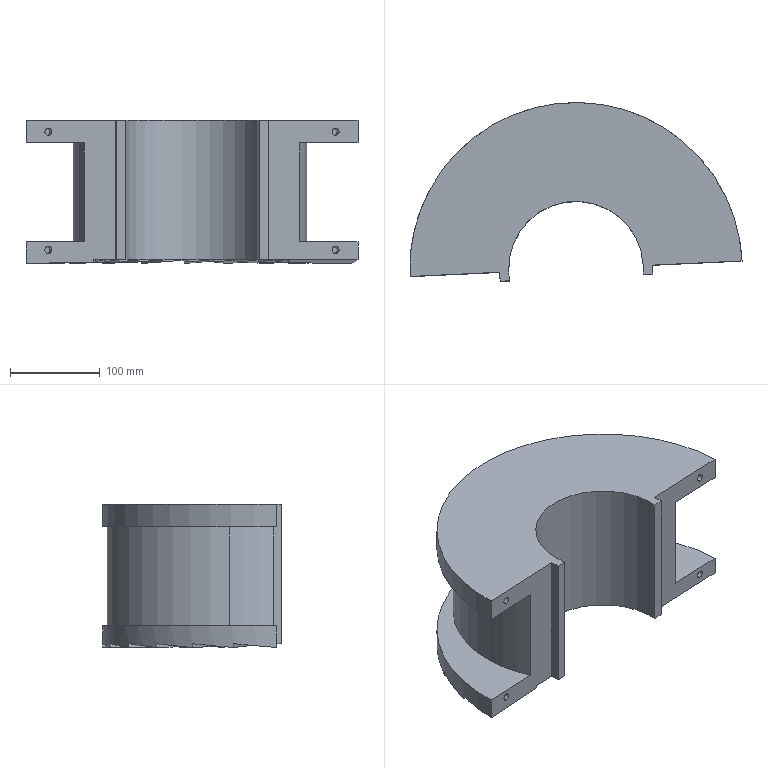Part | SolidWorks | features BaseBody 1 | 1 solid | 65 faces | box 369.799 x 198.951 x 159.255 mm | volume 5445912 mm3 | plane 37 | cylinder 28 | commonest cylinder face diameters 220 x12 8 x8 150 x3 260 x3 370 x2